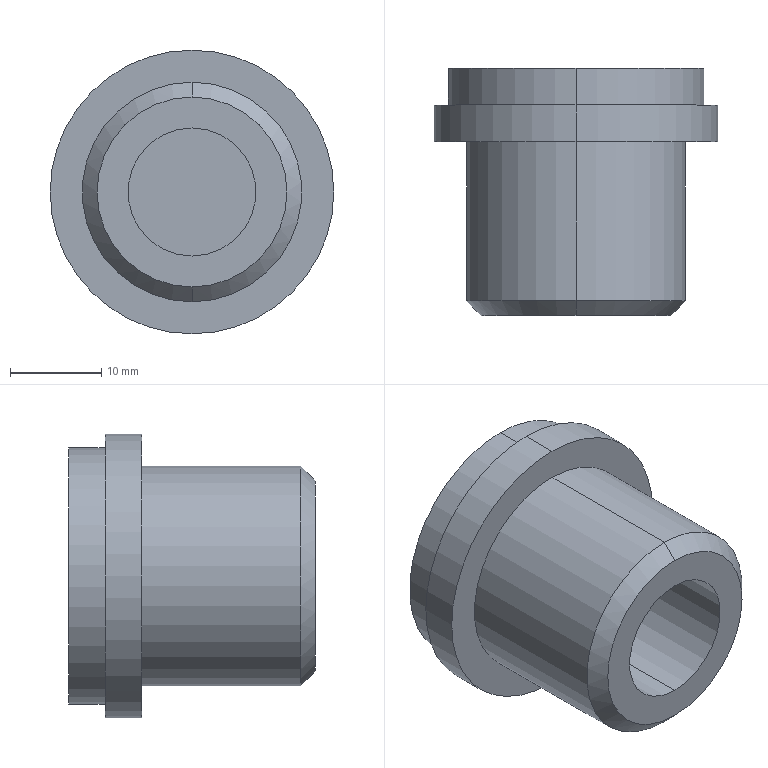Part | SolidWorks | features ICE 4, Extrusion 1, StudWizard 1 | 1 solid | 18 faces | box 31 x 27 x 31 mm | volume 11981 mm3 | cylinder 10 | plane 6 | cone 2 | commonest cylinder face diameters 14 x4 24 x2 28 x2 31 x2
STEP:
#1=CARTESIAN_POINT('',(0.,11.,7.));
#2=VERTEX_POINT('',#1);
#3=CARTESIAN_POINT('',(0.,11.,-7.));
#4=VERTEX_POINT('',#3);
#5=CARTESIAN_POINT('',(0.,11.,0.));
#6=DIRECTION('',(0.,-1.,0.));
#7=DIRECTION('',(0.,0.,-1.));
#8=AXIS2_PLACEMENT_3D('',#5,#6,#7);
#9=CIRCLE('',#8,7.);
#10=EDGE_CURVE('',#2,#4,#9,.T.);
#11=ORIENTED_EDGE('',*,*,#10,.F.);
#12=CARTESIAN_POINT('',(0.,0.,7.));
#13=VERTEX_POINT('',#12);
#14=CARTESIAN_POINT('',(0.,11.,7.));
#15=DIRECTION('',(0.,-1.,0.));
#16=VECTOR('',#15,1000.);
#17=LINE('',#14,#16);
#18=EDGE_CURVE('',#2,#13,#17,.T.);
#19=ORIENTED_EDGE('',*,*,#18,.T.);
#20=CARTESIAN_POINT('',(0.,0.,-7.));
#21=VERTEX_POINT('',#20);
#22=CARTESIAN_POINT('',(0.,0.,0.));
#23=DIRECTION('',(0.,-1.,0.));
#24=DIRECTION('',(0.,0.,-1.));
#25=AXIS2_PLACEMENT_3D('',#22,#23,#24);
#26=CIRCLE('',#25,7.);
#27=EDGE_CURVE('',#13,#21,#26,.T.);
#28=ORIENTED_EDGE('',*,*,#27,.T.);
#29=CARTESIAN_POINT('',(0.,11.,-7.));
#30=DIRECTION('',(0.,-1.,0.));
#31=VECTOR('',#30,1000.);
#32=LINE('',#29,#31);
#33=EDGE_CURVE('',#4,#21,#32,.T.);
#34=ORIENTED_EDGE('',*,*,#33,.F.);
#35=EDGE_LOOP('',(#11,#19,#28,#34));
#36=FACE_OUTER_BOUND('',#35,.T.);
#37=CARTESIAN_POINT('',(0.,11.,0.));
#38=DIRECTION('',(0.,-1.,0.));
#39=DIRECTION('',(0.,0.,-1.));
#40=AXIS2_PLACEMENT_3D('',#37,#38,#39);
#41=CYLINDRICAL_SURFACE('',#40,7.);
#42=ADVANCED_FACE('',(#36),#41,.F.);
#43=CARTESIAN_POINT('',(0.,0.,10.376));
#44=VERTEX_POINT('',#43);
#45=CARTESIAN_POINT('',(0.,0.,-10.376));
#46=VERTEX_POINT('',#45);
#47=CARTESIAN_POINT('',(0.,0.,0.));
#48=DIRECTION('',(0.,1.,0.));
#49=DIRECTION('',(0.,0.,1.));
#50=AXIS2_PLACEMENT_3D('',#47,#48,#49);
#51=CIRCLE('',#50,10.376);
#52=EDGE_CURVE('',#44,#46,#51,.T.);
#53=ORIENTED_EDGE('',*,*,#52,.T.);
#54=CARTESIAN_POINT('',(0.,1.624,-12.));
#55=VERTEX_POINT('',#54);
#56=CARTESIAN_POINT('',(0.,0.,-10.376));
#57=DIRECTION('',(0.,0.7071,-0.7071));
#58=VECTOR('',#57,1000.);
#59=LINE('',#56,#58);
#60=EDGE_CURVE('',#46,#55,#59,.T.);
#61=ORIENTED_EDGE('',*,*,#60,.T.);
#62=CARTESIAN_POINT('',(0.,1.624,12.));
#63=VERTEX_POINT('',#62);
#64=CARTESIAN_POINT('',(0.,1.624,0.));
#65=DIRECTION('',(0.,1.,0.));
#66=DIRECTION('',(0.,0.,1.));
#67=AXIS2_PLACEMENT_3D('',#64,#65,#66);
#68=CIRCLE('',#67,12.);
#69=EDGE_CURVE('',#63,#55,#68,.T.);
#70=ORIENTED_EDGE('',*,*,#69,.F.);
#71=CARTESIAN_POINT('',(0.,0.,10.376));
#72=DIRECTION('',(0.,0.7071,0.7071));
#73=VECTOR('',#72,1000.);
#74=LINE('',#71,#73);
#75=EDGE_CURVE('',#44,#63,#74,.T.);
#76=ORIENTED_EDGE('',*,*,#75,.F.);
#77=EDGE_LOOP('',(#53,#61,#70,#76));
#78=FACE_OUTER_BOUND('',#77,.T.);
#79=CARTESIAN_POINT('',(0.,0.,0.));
#80=DIRECTION('',(0.,1.,0.));
#81=DIRECTION('',(0.,0.,1.));
#82=AXIS2_PLACEMENT_3D('',#79,#80,#81);
#83=CONICAL_SURFACE('',#82,10.376,0.7854);
#84=ADVANCED_FACE('',(#78),#83,.T.);
#85=ORIENTED_EDGE('',*,*,#69,.T.);
#86=CARTESIAN_POINT('',(0.,19.,-12.));
#87=VERTEX_POINT('',#86);
#88=CARTESIAN_POINT('',(0.,0.,-12.));
#89=DIRECTION('',(0.,1.,0.));
#90=VECTOR('',#89,1000.);
#91=LINE('',#88,#90);
#92=EDGE_CURVE('',#55,#87,#91,.T.);
#93=ORIENTED_EDGE('',*,*,#92,.T.);
#94=CARTESIAN_POINT('',(0.,19.,12.));
#95=VERTEX_POINT('',#94);
#96=CARTESIAN_POINT('',(0.,19.,0.));
#97=DIRECTION('',(0.,1.,0.));
#98=DIRECTION('',(0.,0.,1.));
#99=AXIS2_PLACEMENT_3D('',#96,#97,#98);
#100=CIRCLE('',#99,12.);
#101=EDGE_CURVE('',#95,#87,#100,.T.);
#102=ORIENTED_EDGE('',*,*,#101,.F.);
#103=CARTESIAN_POINT('',(0.,0.,12.));
#104=DIRECTION('',(0.,1.,0.));
#105=VECTOR('',#104,1000.);
#106=LINE('',#103,#105);
#107=EDGE_CURVE('',#63,#95,#106,.T.);
#108=ORIENTED_EDGE('',*,*,#107,.F.);
#109=EDGE_LOOP('',(#85,#93,#102,#108));
#110=FACE_OUTER_BOUND('',#109,.T.);
#111=CARTESIAN_POINT('',(0.,0.,0.));
#112=DIRECTION('',(0.,1.,0.));
#113=DIRECTION('',(0.,0.,1.));
#114=AXIS2_PLACEMENT_3D('',#111,#112,#113);
#115=CYLINDRICAL_SURFACE('',#114,12.);
#116=ADVANCED_FACE('',(#110),#115,.T.);
#117=CARTESIAN_POINT('',(0.,25.,-7.));
#118=VERTEX_POINT('',#117);
#119=CARTESIAN_POINT('',(0.,25.,7.));
#120=VERTEX_POINT('',#119);
#121=CARTESIAN_POINT('',(0.,25.,0.));
#122=DIRECTION('',(0.,1.,0.));
#123=DIRECTION('',(0.,0.,1.));
#124=AXIS2_PLACEMENT_3D('',#121,#122,#123);
#125=CIRCLE('',#124,7.);
#126=EDGE_CURVE('',#118,#120,#125,.T.);
#127=ORIENTED_EDGE('',*,*,#126,.F.);
#128=CARTESIAN_POINT('',(0.,27.,-7.));
#129=VERTEX_POINT('',#128);
#130=CARTESIAN_POINT('',(0.,25.,-7.));
#131=DIRECTION('',(0.,1.,0.));
#132=VECTOR('',#131,1000.);
#133=LINE('',#130,#132);
#134=EDGE_CURVE('',#118,#129,#133,.T.);
#135=ORIENTED_EDGE('',*,*,#134,.T.);
#136=CARTESIAN_POINT('',(0.,27.,7.));
#137=VERTEX_POINT('',#136);
#138=CARTESIAN_POINT('',(0.,27.,0.));
#139=DIRECTION('',(0.,1.,0.));
#140=DIRECTION('',(0.,0.,1.));
#141=AXIS2_PLACEMENT_3D('',#138,#139,#140);
#142=CIRCLE('',#141,7.);
#143=EDGE_CURVE('',#129,#137,#142,.T.);
#144=ORIENTED_EDGE('',*,*,#143,.T.);
#145=CARTESIAN_POINT('',(0.,25.,7.));
#146=DIRECTION('',(0.,1.,0.));
#147=VECTOR('',#146,1000.);
#148=LINE('',#145,#147);
#149=EDGE_CURVE('',#120,#137,#148,.T.);
#150=ORIENTED_EDGE('',*,*,#149,.F.);
#151=EDGE_LOOP('',(#127,#135,#144,#150));
#152=FACE_OUTER_BOUND('',#151,.T.);
#153=CARTESIAN_POINT('',(0.,25.,0.));
#154=DIRECTION('',(0.,1.,0.));
#155=DIRECTION('',(0.,0.,1.));
#156=AXIS2_PLACEMENT_3D('',#153,#154,#155);
#157=CYLINDRICAL_SURFACE('',#156,7.);
#158=ADVANCED_FACE('',(#152),#157,.F.);
#159=CARTESIAN_POINT('',(0.,27.,14.));
#160=VERTEX_POINT('',#159);
#161=CARTESIAN_POINT('',(0.,27.,-14.));
#162=VERTEX_POINT('',#161);
#163=CARTESIAN_POINT('',(0.,27.,0.));
#164=DIRECTION('',(0.,1.,0.));
#165=DIRECTION('',(0.,0.,1.));
#166=AXIS2_PLACEMENT_3D('',#163,#164,#165);
#167=CIRCLE('',#166,14.);
#168=EDGE_CURVE('',#160,#162,#167,.T.);
#169=ORIENTED_EDGE('',*,*,#168,.F.);
#170=CARTESIAN_POINT('',(0.,23.,14.));
#171=VERTEX_POINT('',#170);
#172=CARTESIAN_POINT('',(0.,27.,14.));
#173=DIRECTION('',(0.,-1.,0.));
#174=VECTOR('',#173,1000.);
#175=LINE('',#172,#174);
#176=EDGE_CURVE('',#160,#171,#175,.T.);
#177=ORIENTED_EDGE('',*,*,#176,.T.);
#178=CARTESIAN_POINT('',(0.,23.,-14.));
#179=VERTEX_POINT('',#178);
#180=CARTESIAN_POINT('',(0.,23.,0.));
#181=DIRECTION('',(0.,1.,0.));
#182=DIRECTION('',(0.,0.,1.));
#183=AXIS2_PLACEMENT_3D('',#180,#181,#182);
#184=CIRCLE('',#183,14.);
#185=EDGE_CURVE('',#171,#179,#184,.T.);
#186=ORIENTED_EDGE('',*,*,#185,.T.);
#187=CARTESIAN_POINT('',(0.,27.,-14.));
#188=DIRECTION('',(0.,-1.,0.));
#189=VECTOR('',#188,1000.);
#190=LINE('',#187,#189);
#191=EDGE_CURVE('',#162,#179,#190,.T.);
#192=ORIENTED_EDGE('',*,*,#191,.F.);
#193=EDGE_LOOP('',(#169,#177,#186,#192));
#194=FACE_OUTER_BOUND('',#193,.T.);
#195=CARTESIAN_POINT('',(0.,27.,0.));
#196=DIRECTION('',(0.,-1.,0.));
#197=DIRECTION('',(0.,0.,-1.));
#198=AXIS2_PLACEMENT_3D('',#195,#196,#197);
#199=CYLINDRICAL_SURFACE('',#198,14.);
#200=ADVANCED_FACE('',(#194),#199,.T.);
#201=CARTESIAN_POINT('',(0.,23.,15.5));
#202=VERTEX_POINT('',#201);
#203=CARTESIAN_POINT('',(0.,23.,-15.5));
#204=VERTEX_POINT('',#203);
#205=CARTESIAN_POINT('',(0.,23.,0.));
#206=DIRECTION('',(0.,1.,0.));
#207=DIRECTION('',(0.,0.,1.));
#208=AXIS2_PLACEMENT_3D('',#205,#206,#207);
#209=CIRCLE('',#208,15.5);
#210=EDGE_CURVE('',#202,#204,#209,.T.);
#211=ORIENTED_EDGE('',*,*,#210,.F.);
#212=CARTESIAN_POINT('',(0.,19.,15.5));
#213=VERTEX_POINT('',#212);
#214=CARTESIAN_POINT('',(0.,23.,15.5));
#215=DIRECTION('',(0.,-1.,0.));
#216=VECTOR('',#215,1000.);
#217=LINE('',#214,#216);
#218=EDGE_CURVE('',#202,#213,#217,.T.);
#219=ORIENTED_EDGE('',*,*,#218,.T.);
#220=CARTESIAN_POINT('',(0.,19.,-15.5));
#221=VERTEX_POINT('',#220);
#222=CARTESIAN_POINT('',(0.,19.,0.));
#223=DIRECTION('',(0.,1.,0.));
#224=DIRECTION('',(0.,0.,1.));
#225=AXIS2_PLACEMENT_3D('',#222,#223,#224);
#226=CIRCLE('',#225,15.5);
#227=EDGE_CURVE('',#213,#221,#226,.T.);
#228=ORIENTED_EDGE('',*,*,#227,.T.);
#229=CARTESIAN_POINT('',(0.,23.,-15.5));
#230=DIRECTION('',(0.,-1.,0.));
#231=VECTOR('',#230,1000.);
#232=LINE('',#229,#231);
#233=EDGE_CURVE('',#204,#221,#232,.T.);
#234=ORIENTED_EDGE('',*,*,#233,.F.);
#235=EDGE_LOOP('',(#211,#219,#228,#234));
#236=FACE_OUTER_BOUND('',#235,.T.);
#237=CARTESIAN_POINT('',(0.,23.,0.));
#238=DIRECTION('',(0.,-1.,0.));
#239=DIRECTION('',(0.,0.,-1.));
#240=AXIS2_PLACEMENT_3D('',#237,#238,#239);
#241=CYLINDRICAL_SURFACE('',#240,15.5);
#242=ADVANCED_FACE('',(#236),#241,.T.);
#243=ORIENTED_EDGE('',*,*,#218,.F.);
#244=CARTESIAN_POINT('',(0.,23.,0.));
#245=DIRECTION('',(0.,1.,0.));
#246=DIRECTION('',(0.,0.,1.));
#247=AXIS2_PLACEMENT_3D('',#244,#245,#246);
#248=CIRCLE('',#247,15.5);
#249=EDGE_CURVE('',#204,#202,#248,.T.);
#250=ORIENTED_EDGE('',*,*,#249,.F.);
#251=ORIENTED_EDGE('',*,*,#233,.T.);
#252=CARTESIAN_POINT('',(0.,19.,0.));
#253=DIRECTION('',(0.,1.,0.));
#254=DIRECTION('',(0.,0.,1.));
#255=AXIS2_PLACEMENT_3D('',#252,#253,#254);
#256=CIRCLE('',#255,15.5);
#257=EDGE_CURVE('',#221,#213,#256,.T.);
#258=ORIENTED_EDGE('',*,*,#257,.T.);
#259=EDGE_LOOP('',(#243,#250,#251,#258));
#260=FACE_OUTER_BOUND('',#259,.T.);
#261=CARTESIAN_POINT('',(0.,23.,0.));
#262=DIRECTION('',(0.,-1.,0.));
#263=DIRECTION('',(0.,0.,-1.));
#264=AXIS2_PLACEMENT_3D('',#261,#262,#263);
#265=CYLINDRICAL_SURFACE('',#264,15.5);
#266=ADVANCED_FACE('',(#260),#265,.T.);
#267=CARTESIAN_POINT('',(0.,23.,0.));
#268=DIRECTION('',(0.,1.,0.));
#269=DIRECTION('',(0.,0.,1.));
#270=AXIS2_PLACEMENT_3D('',#267,#268,#269);
#271=CIRCLE('',#270,14.);
#272=EDGE_CURVE('',#179,#171,#271,.T.);
#273=ORIENTED_EDGE('',*,*,#272,.F.);
#274=ORIENTED_EDGE('',*,*,#185,.F.);
#275=EDGE_LOOP('',(#273,#274));
#276=FACE_BOUND('',#275,.T.);
#277=ORIENTED_EDGE('',*,*,#249,.T.);
#278=ORIENTED_EDGE('',*,*,#210,.T.);
#279=EDGE_LOOP('',(#277,#278));
#280=FACE_OUTER_BOUND('',#279,.T.);
#281=CARTESIAN_POINT('',(0.,23.,0.));
#282=DIRECTION('',(0.,1.,0.));
#283=DIRECTION('',(0.,0.,1.));
#284=AXIS2_PLACEMENT_3D('',#281,#282,#283);
#285=PLANE('',#284);
#286=ADVANCED_FACE('',(#276,#280),#285,.T.);
#287=ORIENTED_EDGE('',*,*,#257,.F.);
#288=ORIENTED_EDGE('',*,*,#227,.F.);
#289=EDGE_LOOP('',(#287,#288));
#290=FACE_OUTER_BOUND('',#289,.T.);
#291=ORIENTED_EDGE('',*,*,#101,.T.);
#292=CARTESIAN_POINT('',(0.,19.,0.));
#293=DIRECTION('',(0.,1.,0.));
#294=DIRECTION('',(0.,0.,1.));
#295=AXIS2_PLACEMENT_3D('',#292,#293,#294);
#296=CIRCLE('',#295,12.);
#297=EDGE_CURVE('',#87,#95,#296,.T.);
#298=ORIENTED_EDGE('',*,*,#297,.T.);
#299=EDGE_LOOP('',(#291,#298));
#300=FACE_BOUND('',#299,.T.);
#301=CARTESIAN_POINT('',(0.,19.,0.));
#302=DIRECTION('',(0.,1.,0.));
#303=DIRECTION('',(0.,0.,1.));
#304=AXIS2_PLACEMENT_3D('',#301,#302,#303);
#305=PLANE('',#304);
#306=ADVANCED_FACE('',(#290,#300),#305,.F.);
#307=ORIENTED_EDGE('',*,*,#176,.F.);
#308=CARTESIAN_POINT('',(0.,27.,0.));
#309=DIRECTION('',(0.,1.,0.));
#310=DIRECTION('',(0.,0.,1.));
#311=AXIS2_PLACEMENT_3D('',#308,#309,#310);
#312=CIRCLE('',#311,14.);
#313=EDGE_CURVE('',#162,#160,#312,.T.);
#314=ORIENTED_EDGE('',*,*,#313,.F.);
#315=ORIENTED_EDGE('',*,*,#191,.T.);
#316=ORIENTED_EDGE('',*,*,#272,.T.);
#317=EDGE_LOOP('',(#307,#314,#315,#316));
#318=FACE_OUTER_BOUND('',#317,.T.);
#319=CARTESIAN_POINT('',(0.,27.,0.));
#320=DIRECTION('',(0.,-1.,0.));
#321=DIRECTION('',(0.,0.,-1.));
#322=AXIS2_PLACEMENT_3D('',#319,#320,#321);
#323=CYLINDRICAL_SURFACE('',#322,14.);
#324=ADVANCED_FACE('',(#318),#323,.T.);
#325=CARTESIAN_POINT('',(0.,27.,0.));
#326=DIRECTION('',(0.,1.,0.));
#327=DIRECTION('',(0.,0.,1.));
#328=AXIS2_PLACEMENT_3D('',#325,#326,#327);
#329=CIRCLE('',#328,7.);
#330=EDGE_CURVE('',#137,#129,#329,.T.);
#331=ORIENTED_EDGE('',*,*,#330,.F.);
#332=ORIENTED_EDGE('',*,*,#143,.F.);
#333=EDGE_LOOP('',(#331,#332));
#334=FACE_BOUND('',#333,.T.);
#335=ORIENTED_EDGE('',*,*,#313,.T.);
#336=ORIENTED_EDGE('',*,*,#168,.T.);
#337=EDGE_LOOP('',(#335,#336));
#338=FACE_OUTER_BOUND('',#337,.T.);
#339=CARTESIAN_POINT('',(0.,27.,0.));
#340=DIRECTION('',(0.,1.,0.));
#341=DIRECTION('',(0.,0.,1.));
#342=AXIS2_PLACEMENT_3D('',#339,#340,#341);
#343=PLANE('',#342);
#344=ADVANCED_FACE('',(#334,#338),#343,.T.);
#345=ORIENTED_EDGE('',*,*,#134,.F.);
#346=CARTESIAN_POINT('',(0.,25.,0.));
#347=DIRECTION('',(0.,1.,0.));
#348=DIRECTION('',(0.,0.,1.));
#349=AXIS2_PLACEMENT_3D('',#346,#347,#348);
#350=CIRCLE('',#349,7.);
#351=EDGE_CURVE('',#120,#118,#350,.T.);
#352=ORIENTED_EDGE('',*,*,#351,.F.);
#353=ORIENTED_EDGE('',*,*,#149,.T.);
#354=ORIENTED_EDGE('',*,*,#330,.T.);
#355=EDGE_LOOP('',(#345,#352,#353,#354));
#356=FACE_OUTER_BOUND('',#355,.T.);
#357=CARTESIAN_POINT('',(0.,25.,0.));
#358=DIRECTION('',(0.,1.,0.));
#359=DIRECTION('',(0.,0.,1.));
#360=AXIS2_PLACEMENT_3D('',#357,#358,#359);
#361=CYLINDRICAL_SURFACE('',#360,7.);
#362=ADVANCED_FACE('',(#356),#361,.F.);
#363=ORIENTED_EDGE('',*,*,#351,.T.);
#364=ORIENTED_EDGE('',*,*,#126,.T.);
#365=EDGE_LOOP('',(#363,#364));
#366=FACE_OUTER_BOUND('',#365,.T.);
#367=CARTESIAN_POINT('',(0.,25.,0.));
#368=DIRECTION('',(0.,1.,0.));
#369=DIRECTION('',(0.,0.,1.));
#370=AXIS2_PLACEMENT_3D('',#367,#368,#369);
#371=PLANE('',#370);
#372=ADVANCED_FACE('',(#366),#371,.T.);
#373=ORIENTED_EDGE('',*,*,#92,.F.);
#374=CARTESIAN_POINT('',(0.,1.624,0.));
#375=DIRECTION('',(0.,1.,0.));
#376=DIRECTION('',(0.,0.,1.));
#377=AXIS2_PLACEMENT_3D('',#374,#375,#376);
#378=CIRCLE('',#377,12.);
#379=EDGE_CURVE('',#55,#63,#378,.T.);
#380=ORIENTED_EDGE('',*,*,#379,.T.);
#381=ORIENTED_EDGE('',*,*,#107,.T.);
#382=ORIENTED_EDGE('',*,*,#297,.F.);
#383=EDGE_LOOP('',(#373,#380,#381,#382));
#384=FACE_OUTER_BOUND('',#383,.T.);
#385=CARTESIAN_POINT('',(0.,0.,0.));
#386=DIRECTION('',(0.,1.,0.));
#387=DIRECTION('',(0.,0.,1.));
#388=AXIS2_PLACEMENT_3D('',#385,#386,#387);
#389=CYLINDRICAL_SURFACE('',#388,12.);
#390=ADVANCED_FACE('',(#384),#389,.T.);
#391=ORIENTED_EDGE('',*,*,#60,.F.);
#392=CARTESIAN_POINT('',(0.,0.,0.));
#393=DIRECTION('',(0.,1.,0.));
#394=DIRECTION('',(0.,0.,1.));
#395=AXIS2_PLACEMENT_3D('',#392,#393,#394);
#396=CIRCLE('',#395,10.376);
#397=EDGE_CURVE('',#46,#44,#396,.T.);
#398=ORIENTED_EDGE('',*,*,#397,.T.);
#399=ORIENTED_EDGE('',*,*,#75,.T.);
#400=ORIENTED_EDGE('',*,*,#379,.F.);
#401=EDGE_LOOP('',(#391,#398,#399,#400));
#402=FACE_OUTER_BOUND('',#401,.T.);
#403=CARTESIAN_POINT('',(0.,0.,0.));
#404=DIRECTION('',(0.,1.,0.));
#405=DIRECTION('',(0.,0.,1.));
#406=AXIS2_PLACEMENT_3D('',#403,#404,#405);
#407=CONICAL_SURFACE('',#406,10.376,0.7854);
#408=ADVANCED_FACE('',(#402),#407,.T.);
#409=CARTESIAN_POINT('',(0.,11.,0.));
#410=DIRECTION('',(0.,-1.,0.));
#411=DIRECTION('',(0.,0.,-1.));
#412=AXIS2_PLACEMENT_3D('',#409,#410,#411);
#413=CIRCLE('',#412,7.);
#414=EDGE_CURVE('',#4,#2,#413,.T.);
#415=ORIENTED_EDGE('',*,*,#414,.T.);
#416=ORIENTED_EDGE('',*,*,#10,.T.);
#417=EDGE_LOOP('',(#415,#416));
#418=FACE_OUTER_BOUND('',#417,.T.);
#419=CARTESIAN_POINT('',(0.,11.,0.));
#420=DIRECTION('',(0.,-1.,0.));
#421=DIRECTION('',(0.,0.,-1.));
#422=AXIS2_PLACEMENT_3D('',#419,#420,#421);
#423=PLANE('',#422);
#424=ADVANCED_FACE('',(#418),#423,.T.);
#425=ORIENTED_EDGE('',*,*,#18,.F.);
#426=ORIENTED_EDGE('',*,*,#414,.F.);
#427=ORIENTED_EDGE('',*,*,#33,.T.);
#428=CARTESIAN_POINT('',(0.,0.,0.));
#429=DIRECTION('',(0.,-1.,0.));
#430=DIRECTION('',(0.,0.,-1.));
#431=AXIS2_PLACEMENT_3D('',#428,#429,#430);
#432=CIRCLE('',#431,7.);
#433=EDGE_CURVE('',#21,#13,#432,.T.);
#434=ORIENTED_EDGE('',*,*,#433,.T.);
#435=EDGE_LOOP('',(#425,#426,#427,#434));
#436=FACE_OUTER_BOUND('',#435,.T.);
#437=CARTESIAN_POINT('',(0.,11.,0.));
#438=DIRECTION('',(0.,-1.,0.));
#439=DIRECTION('',(0.,0.,-1.));
#440=AXIS2_PLACEMENT_3D('',#437,#438,#439);
#441=CYLINDRICAL_SURFACE('',#440,7.);
#442=ADVANCED_FACE('',(#436),#441,.F.);
#443=ORIENTED_EDGE('',*,*,#433,.F.);
#444=ORIENTED_EDGE('',*,*,#27,.F.);
#445=EDGE_LOOP('',(#443,#444));
#446=FACE_BOUND('',#445,.T.);
#447=ORIENTED_EDGE('',*,*,#52,.F.);
#448=ORIENTED_EDGE('',*,*,#397,.F.);
#449=EDGE_LOOP('',(#447,#448));
#450=FACE_OUTER_BOUND('',#449,.T.);
#451=CARTESIAN_POINT('',(0.,0.,0.));
#452=DIRECTION('',(0.,1.,0.));
#453=DIRECTION('',(0.,0.,1.));
#454=AXIS2_PLACEMENT_3D('',#451,#452,#453);
#455=PLANE('',#454);
#456=ADVANCED_FACE('',(#446,#450),#455,.F.);
#457=CLOSED_SHELL('',(#42,#84,#116,#158,#200,#242,#266,#286,#306,#324,#344,#362,#372,#390,#408,#424,#442,#456));
#458=MANIFOLD_SOLID_BREP('',#457);
#459=CARTESIAN_POINT('',(0.,0.,0.));
#460=DIRECTION('',(0.,0.,1.));
#461=DIRECTION('',(1.,0.,0.));
#462=AXIS2_PLACEMENT_3D('',#459,#460,#461);
#463=(LENGTH_UNIT()NAMED_UNIT(*)SI_UNIT(.MILLI.,.METRE.));
#464=UNCERTAINTY_MEASURE_WITH_UNIT(LENGTH_MEASURE(0.00001),#463,'','');
#465=(NAMED_UNIT(*)PLANE_ANGLE_UNIT()SI_UNIT($,.RADIAN.));
#466=(NAMED_UNIT(*)SI_UNIT($,.STERADIAN.)SOLID_ANGLE_UNIT());
#467=(GEOMETRIC_REPRESENTATION_CONTEXT(3)GLOBAL_UNCERTAINTY_ASSIGNED_CONTEXT((#464))GLOBAL_UNIT_ASSIGNED_CONTEXT((#463,#465,#466))REPRESENTATION_CONTEXT('',''));
#468=ADVANCED_BREP_SHAPE_REPRESENTATION('',(#458,#462),#467);